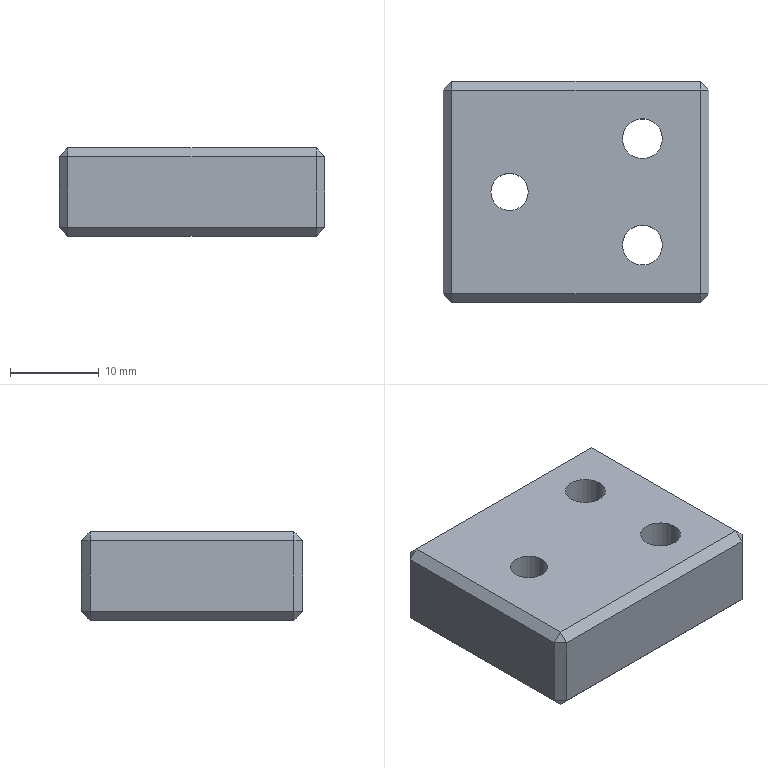Part | STEP file | 04-23 belt tensioning plate | 1 solid | 38 faces | box 30 x 25 x 10 mm | volume 6603 mm3 | plane 28 | cylinder 10 | commonest cylinder face diameters 4.5 x4 8 x4 4.2 x2
STEP:
#1=CARTESIAN_POINT('',(-9.6,0.,10.));
#2=VERTEX_POINT('',#1);
#3=CARTESIAN_POINT('',(-5.4,0.,10.));
#4=VERTEX_POINT('',#3);
#5=CARTESIAN_POINT('',(-7.5,0.,10.));
#6=DIRECTION('',(0.,0.,1.));
#7=DIRECTION('',(1.,0.,0.));
#8=AXIS2_PLACEMENT_3D('',#5,#6,#7);
#9=CIRCLE('',#8,2.1);
#10=EDGE_CURVE('',#2,#4,#9,.T.);
#11=ORIENTED_EDGE('',*,*,#10,.T.);
#12=CARTESIAN_POINT('',(-5.4,0.,0.));
#13=VERTEX_POINT('',#12);
#14=CARTESIAN_POINT('',(-5.4,0.,0.));
#15=DIRECTION('',(0.,0.,-1.));
#16=VECTOR('',#15,1000.);
#17=LINE('',#14,#16);
#18=EDGE_CURVE('',#4,#13,#17,.T.);
#19=ORIENTED_EDGE('',*,*,#18,.T.);
#20=CARTESIAN_POINT('',(-9.6,0.,0.));
#21=VERTEX_POINT('',#20);
#22=CARTESIAN_POINT('',(-7.5,0.,0.));
#23=DIRECTION('',(0.,0.,-1.));
#24=DIRECTION('',(-1.,0.,0.));
#25=AXIS2_PLACEMENT_3D('',#22,#23,#24);
#26=CIRCLE('',#25,2.1);
#27=EDGE_CURVE('',#13,#21,#26,.T.);
#28=ORIENTED_EDGE('',*,*,#27,.T.);
#29=CARTESIAN_POINT('',(-9.6,0.,0.));
#30=DIRECTION('',(0.,0.,-1.));
#31=VECTOR('',#30,1000.);
#32=LINE('',#29,#31);
#33=EDGE_CURVE('',#2,#21,#32,.T.);
#34=ORIENTED_EDGE('',*,*,#33,.F.);
#35=EDGE_LOOP('',(#11,#19,#28,#34));
#36=FACE_OUTER_BOUND('',#35,.T.);
#37=CARTESIAN_POINT('',(-7.5,0.,0.));
#38=DIRECTION('',(0.,0.,-1.));
#39=DIRECTION('',(-1.,0.,0.));
#40=AXIS2_PLACEMENT_3D('',#37,#38,#39);
#41=CYLINDRICAL_SURFACE('',#40,2.1);
#42=ADVANCED_FACE('',(#36),#41,.F.);
#43=CARTESIAN_POINT('',(11.5,6.,4.6));
#44=VERTEX_POINT('',#43);
#45=CARTESIAN_POINT('',(3.5,6.,4.6));
#46=VERTEX_POINT('',#45);
#47=CARTESIAN_POINT('',(7.5,6.,4.6));
#48=DIRECTION('',(0.,0.,-1.));
#49=DIRECTION('',(-1.,0.,0.));
#50=AXIS2_PLACEMENT_3D('',#47,#48,#49);
#51=CIRCLE('',#50,4.);
#52=EDGE_CURVE('',#44,#46,#51,.T.);
#53=ORIENTED_EDGE('',*,*,#52,.F.);
#54=CARTESIAN_POINT('',(11.5,6.,0.));
#55=VERTEX_POINT('',#54);
#56=CARTESIAN_POINT('',(11.5,6.,0.));
#57=DIRECTION('',(0.,0.,-1.));
#58=VECTOR('',#57,1000.);
#59=LINE('',#56,#58);
#60=EDGE_CURVE('',#44,#55,#59,.T.);
#61=ORIENTED_EDGE('',*,*,#60,.T.);
#62=CARTESIAN_POINT('',(3.5,6.,0.));
#63=VERTEX_POINT('',#62);
#64=CARTESIAN_POINT('',(7.5,6.,0.));
#65=DIRECTION('',(0.,0.,-1.));
#66=DIRECTION('',(-1.,0.,0.));
#67=AXIS2_PLACEMENT_3D('',#64,#65,#66);
#68=CIRCLE('',#67,4.);
#69=EDGE_CURVE('',#55,#63,#68,.T.);
#70=ORIENTED_EDGE('',*,*,#69,.T.);
#71=CARTESIAN_POINT('',(3.5,6.,0.));
#72=DIRECTION('',(0.,0.,-1.));
#73=VECTOR('',#72,1000.);
#74=LINE('',#71,#73);
#75=EDGE_CURVE('',#46,#63,#74,.T.);
#76=ORIENTED_EDGE('',*,*,#75,.F.);
#77=EDGE_LOOP('',(#53,#61,#70,#76));
#78=FACE_OUTER_BOUND('',#77,.T.);
#79=CARTESIAN_POINT('',(7.5,6.,0.));
#80=DIRECTION('',(0.,0.,-1.));
#81=DIRECTION('',(-1.,0.,0.));
#82=AXIS2_PLACEMENT_3D('',#79,#80,#81);
#83=CYLINDRICAL_SURFACE('',#82,4.);
#84=ADVANCED_FACE('',(#78),#83,.F.);
#85=CARTESIAN_POINT('',(9.75,6.,10.));
#86=VERTEX_POINT('',#85);
#87=CARTESIAN_POINT('',(5.25,6.,10.));
#88=VERTEX_POINT('',#87);
#89=CARTESIAN_POINT('',(7.5,6.,10.));
#90=DIRECTION('',(0.,0.,-1.));
#91=DIRECTION('',(-1.,0.,0.));
#92=AXIS2_PLACEMENT_3D('',#89,#90,#91);
#93=CIRCLE('',#92,2.25);
#94=EDGE_CURVE('',#86,#88,#93,.T.);
#95=ORIENTED_EDGE('',*,*,#94,.F.);
#96=CARTESIAN_POINT('',(9.75,6.,4.6));
#97=VERTEX_POINT('',#96);
#98=CARTESIAN_POINT('',(9.75,6.,0.));
#99=DIRECTION('',(0.,0.,-1.));
#100=VECTOR('',#99,1000.);
#101=LINE('',#98,#100);
#102=EDGE_CURVE('',#86,#97,#101,.T.);
#103=ORIENTED_EDGE('',*,*,#102,.T.);
#104=CARTESIAN_POINT('',(5.25,6.,4.6));
#105=VERTEX_POINT('',#104);
#106=CARTESIAN_POINT('',(7.5,6.,4.6));
#107=DIRECTION('',(0.,0.,-1.));
#108=DIRECTION('',(-1.,0.,0.));
#109=AXIS2_PLACEMENT_3D('',#106,#107,#108);
#110=CIRCLE('',#109,2.25);
#111=EDGE_CURVE('',#97,#105,#110,.T.);
#112=ORIENTED_EDGE('',*,*,#111,.T.);
#113=CARTESIAN_POINT('',(5.25,6.,0.));
#114=DIRECTION('',(0.,0.,-1.));
#115=VECTOR('',#114,1000.);
#116=LINE('',#113,#115);
#117=EDGE_CURVE('',#88,#105,#116,.T.);
#118=ORIENTED_EDGE('',*,*,#117,.F.);
#119=EDGE_LOOP('',(#95,#103,#112,#118));
#120=FACE_OUTER_BOUND('',#119,.T.);
#121=CARTESIAN_POINT('',(7.5,6.,0.));
#122=DIRECTION('',(0.,0.,-1.));
#123=DIRECTION('',(-1.,0.,0.));
#124=AXIS2_PLACEMENT_3D('',#121,#122,#123);
#125=CYLINDRICAL_SURFACE('',#124,2.25);
#126=ADVANCED_FACE('',(#120),#125,.F.);
#127=CARTESIAN_POINT('',(11.5,-6.,4.6));
#128=VERTEX_POINT('',#127);
#129=CARTESIAN_POINT('',(3.5,-6.,4.6));
#130=VERTEX_POINT('',#129);
#131=CARTESIAN_POINT('',(7.5,-6.,4.6));
#132=DIRECTION('',(0.,0.,-1.));
#133=DIRECTION('',(-1.,0.,0.));
#134=AXIS2_PLACEMENT_3D('',#131,#132,#133);
#135=CIRCLE('',#134,4.);
#136=EDGE_CURVE('',#128,#130,#135,.T.);
#137=ORIENTED_EDGE('',*,*,#136,.F.);
#138=CARTESIAN_POINT('',(11.5,-6.,0.));
#139=VERTEX_POINT('',#138);
#140=CARTESIAN_POINT('',(11.5,-6.,0.));
#141=DIRECTION('',(0.,0.,-1.));
#142=VECTOR('',#141,1000.);
#143=LINE('',#140,#142);
#144=EDGE_CURVE('',#128,#139,#143,.T.);
#145=ORIENTED_EDGE('',*,*,#144,.T.);
#146=CARTESIAN_POINT('',(3.5,-6.,0.));
#147=VERTEX_POINT('',#146);
#148=CARTESIAN_POINT('',(7.5,-6.,0.));
#149=DIRECTION('',(0.,0.,-1.));
#150=DIRECTION('',(-1.,0.,0.));
#151=AXIS2_PLACEMENT_3D('',#148,#149,#150);
#152=CIRCLE('',#151,4.);
#153=EDGE_CURVE('',#139,#147,#152,.T.);
#154=ORIENTED_EDGE('',*,*,#153,.T.);
#155=CARTESIAN_POINT('',(3.5,-6.,0.));
#156=DIRECTION('',(0.,0.,-1.));
#157=VECTOR('',#156,1000.);
#158=LINE('',#155,#157);
#159=EDGE_CURVE('',#130,#147,#158,.T.);
#160=ORIENTED_EDGE('',*,*,#159,.F.);
#161=EDGE_LOOP('',(#137,#145,#154,#160));
#162=FACE_OUTER_BOUND('',#161,.T.);
#163=CARTESIAN_POINT('',(7.5,-6.,0.));
#164=DIRECTION('',(0.,0.,-1.));
#165=DIRECTION('',(-1.,0.,0.));
#166=AXIS2_PLACEMENT_3D('',#163,#164,#165);
#167=CYLINDRICAL_SURFACE('',#166,4.);
#168=ADVANCED_FACE('',(#162),#167,.F.);
#169=CARTESIAN_POINT('',(9.75,-6.,10.));
#170=VERTEX_POINT('',#169);
#171=CARTESIAN_POINT('',(5.25,-6.,10.));
#172=VERTEX_POINT('',#171);
#173=CARTESIAN_POINT('',(7.5,-6.,10.));
#174=DIRECTION('',(0.,0.,-1.));
#175=DIRECTION('',(-1.,0.,0.));
#176=AXIS2_PLACEMENT_3D('',#173,#174,#175);
#177=CIRCLE('',#176,2.25);
#178=EDGE_CURVE('',#170,#172,#177,.T.);
#179=ORIENTED_EDGE('',*,*,#178,.F.);
#180=CARTESIAN_POINT('',(9.75,-6.,4.6));
#181=VERTEX_POINT('',#180);
#182=CARTESIAN_POINT('',(9.75,-6.,0.));
#183=DIRECTION('',(0.,0.,-1.));
#184=VECTOR('',#183,1000.);
#185=LINE('',#182,#184);
#186=EDGE_CURVE('',#170,#181,#185,.T.);
#187=ORIENTED_EDGE('',*,*,#186,.T.);
#188=CARTESIAN_POINT('',(5.25,-6.,4.6));
#189=VERTEX_POINT('',#188);
#190=CARTESIAN_POINT('',(7.5,-6.,4.6));
#191=DIRECTION('',(0.,0.,-1.));
#192=DIRECTION('',(-1.,0.,0.));
#193=AXIS2_PLACEMENT_3D('',#190,#191,#192);
#194=CIRCLE('',#193,2.25);
#195=EDGE_CURVE('',#181,#189,#194,.T.);
#196=ORIENTED_EDGE('',*,*,#195,.T.);
#197=CARTESIAN_POINT('',(5.25,-6.,0.));
#198=DIRECTION('',(0.,0.,-1.));
#199=VECTOR('',#198,1000.);
#200=LINE('',#197,#199);
#201=EDGE_CURVE('',#172,#189,#200,.T.);
#202=ORIENTED_EDGE('',*,*,#201,.F.);
#203=EDGE_LOOP('',(#179,#187,#196,#202));
#204=FACE_OUTER_BOUND('',#203,.T.);
#205=CARTESIAN_POINT('',(7.5,-6.,0.));
#206=DIRECTION('',(0.,0.,-1.));
#207=DIRECTION('',(-1.,0.,0.));
#208=AXIS2_PLACEMENT_3D('',#205,#206,#207);
#209=CYLINDRICAL_SURFACE('',#208,2.25);
#210=ADVANCED_FACE('',(#204),#209,.F.);
#211=CARTESIAN_POINT('',(15.,11.5,9.));
#212=VERTEX_POINT('',#211);
#213=CARTESIAN_POINT('',(15.,-11.5,9.));
#214=VERTEX_POINT('',#213);
#215=CARTESIAN_POINT('',(15.,-12.5,9.));
#216=DIRECTION('',(0.,-1.,0.));
#217=VECTOR('',#216,1000.);
#218=LINE('',#215,#217);
#219=EDGE_CURVE('',#212,#214,#218,.T.);
#220=ORIENTED_EDGE('',*,*,#219,.T.);
#221=CARTESIAN_POINT('',(15.,-11.5,1.));
#222=VERTEX_POINT('',#221);
#223=CARTESIAN_POINT('',(15.,-11.5,10.));
#224=DIRECTION('',(0.,0.,-1.));
#225=VECTOR('',#224,1000.);
#226=LINE('',#223,#225);
#227=EDGE_CURVE('',#214,#222,#226,.T.);
#228=ORIENTED_EDGE('',*,*,#227,.T.);
#229=CARTESIAN_POINT('',(15.,11.5,1.));
#230=VERTEX_POINT('',#229);
#231=CARTESIAN_POINT('',(15.,12.5,1.));
#232=DIRECTION('',(0.,1.,0.));
#233=VECTOR('',#232,1000.);
#234=LINE('',#231,#233);
#235=EDGE_CURVE('',#222,#230,#234,.T.);
#236=ORIENTED_EDGE('',*,*,#235,.T.);
#237=CARTESIAN_POINT('',(15.,11.5,10.));
#238=DIRECTION('',(0.,0.,1.));
#239=VECTOR('',#238,1000.);
#240=LINE('',#237,#239);
#241=EDGE_CURVE('',#230,#212,#240,.T.);
#242=ORIENTED_EDGE('',*,*,#241,.T.);
#243=EDGE_LOOP('',(#220,#228,#236,#242));
#244=FACE_OUTER_BOUND('',#243,.T.);
#245=CARTESIAN_POINT('',(15.,12.5,10.));
#246=DIRECTION('',(-1.,0.,0.));
#247=DIRECTION('',(0.,-1.,0.));
#248=AXIS2_PLACEMENT_3D('',#245,#246,#247);
#249=PLANE('',#248);
#250=ADVANCED_FACE('',(#244),#249,.F.);
#251=CARTESIAN_POINT('',(-14.,12.5,9.));
#252=VERTEX_POINT('',#251);
#253=CARTESIAN_POINT('',(14.,12.5,9.));
#254=VERTEX_POINT('',#253);
#255=CARTESIAN_POINT('',(15.,12.5,9.));
#256=DIRECTION('',(1.,0.,0.));
#257=VECTOR('',#256,1000.);
#258=LINE('',#255,#257);
#259=EDGE_CURVE('',#252,#254,#258,.T.);
#260=ORIENTED_EDGE('',*,*,#259,.T.);
#261=CARTESIAN_POINT('',(14.,12.5,1.));
#262=VERTEX_POINT('',#261);
#263=CARTESIAN_POINT('',(14.,12.5,10.));
#264=DIRECTION('',(0.,0.,-1.));
#265=VECTOR('',#264,1000.);
#266=LINE('',#263,#265);
#267=EDGE_CURVE('',#254,#262,#266,.T.);
#268=ORIENTED_EDGE('',*,*,#267,.T.);
#269=CARTESIAN_POINT('',(-14.,12.5,1.));
#270=VERTEX_POINT('',#269);
#271=CARTESIAN_POINT('',(-15.,12.5,1.));
#272=DIRECTION('',(-1.,0.,0.));
#273=VECTOR('',#272,1000.);
#274=LINE('',#271,#273);
#275=EDGE_CURVE('',#262,#270,#274,.T.);
#276=ORIENTED_EDGE('',*,*,#275,.T.);
#277=CARTESIAN_POINT('',(-14.,12.5,10.));
#278=DIRECTION('',(0.,0.,1.));
#279=VECTOR('',#278,1000.);
#280=LINE('',#277,#279);
#281=EDGE_CURVE('',#270,#252,#280,.T.);
#282=ORIENTED_EDGE('',*,*,#281,.T.);
#283=EDGE_LOOP('',(#260,#268,#276,#282));
#284=FACE_OUTER_BOUND('',#283,.T.);
#285=CARTESIAN_POINT('',(-15.,12.5,10.));
#286=DIRECTION('',(0.,-1.,0.));
#287=DIRECTION('',(0.,0.,-1.));
#288=AXIS2_PLACEMENT_3D('',#285,#286,#287);
#289=PLANE('',#288);
#290=ADVANCED_FACE('',(#284),#289,.F.);
#291=CARTESIAN_POINT('',(-15.,-11.5,1.));
#292=VERTEX_POINT('',#291);
#293=CARTESIAN_POINT('',(-15.,-11.5,9.));
#294=VERTEX_POINT('',#293);
#295=CARTESIAN_POINT('',(-15.,-11.5,10.));
#296=DIRECTION('',(0.,0.,1.));
#297=VECTOR('',#296,1000.);
#298=LINE('',#295,#297);
#299=EDGE_CURVE('',#292,#294,#298,.T.);
#300=ORIENTED_EDGE('',*,*,#299,.T.);
#301=CARTESIAN_POINT('',(-15.,11.5,9.));
#302=VERTEX_POINT('',#301);
#303=CARTESIAN_POINT('',(-15.,12.5,9.));
#304=DIRECTION('',(0.,1.,0.));
#305=VECTOR('',#304,1000.);
#306=LINE('',#303,#305);
#307=EDGE_CURVE('',#294,#302,#306,.T.);
#308=ORIENTED_EDGE('',*,*,#307,.T.);
#309=CARTESIAN_POINT('',(-15.,11.5,1.));
#310=VERTEX_POINT('',#309);
#311=CARTESIAN_POINT('',(-15.,11.5,10.));
#312=DIRECTION('',(0.,0.,-1.));
#313=VECTOR('',#312,1000.);
#314=LINE('',#311,#313);
#315=EDGE_CURVE('',#302,#310,#314,.T.);
#316=ORIENTED_EDGE('',*,*,#315,.T.);
#317=CARTESIAN_POINT('',(-15.,12.5,1.));
#318=DIRECTION('',(0.,-1.,0.));
#319=VECTOR('',#318,1000.);
#320=LINE('',#317,#319);
#321=EDGE_CURVE('',#310,#292,#320,.T.);
#322=ORIENTED_EDGE('',*,*,#321,.T.);
#323=EDGE_LOOP('',(#300,#308,#316,#322));
#324=FACE_OUTER_BOUND('',#323,.T.);
#325=CARTESIAN_POINT('',(-15.,12.5,10.));
#326=DIRECTION('',(1.,0.,0.));
#327=DIRECTION('',(0.,1.,0.));
#328=AXIS2_PLACEMENT_3D('',#325,#326,#327);
#329=PLANE('',#328);
#330=ADVANCED_FACE('',(#324),#329,.F.);
#331=CARTESIAN_POINT('',(14.,-12.5,1.));
#332=VERTEX_POINT('',#331);
#333=CARTESIAN_POINT('',(14.,-12.5,9.));
#334=VERTEX_POINT('',#333);
#335=CARTESIAN_POINT('',(14.,-12.5,10.));
#336=DIRECTION('',(0.,0.,1.));
#337=VECTOR('',#336,1000.);
#338=LINE('',#335,#337);
#339=EDGE_CURVE('',#332,#334,#338,.T.);
#340=ORIENTED_EDGE('',*,*,#339,.T.);
#341=CARTESIAN_POINT('',(-14.,-12.5,9.));
#342=VERTEX_POINT('',#341);
#343=CARTESIAN_POINT('',(-15.,-12.5,9.));
#344=DIRECTION('',(-1.,0.,0.));
#345=VECTOR('',#344,1000.);
#346=LINE('',#343,#345);
#347=EDGE_CURVE('',#334,#342,#346,.T.);
#348=ORIENTED_EDGE('',*,*,#347,.T.);
#349=CARTESIAN_POINT('',(-14.,-12.5,1.));
#350=VERTEX_POINT('',#349);
#351=CARTESIAN_POINT('',(-14.,-12.5,10.));
#352=DIRECTION('',(0.,0.,-1.));
#353=VECTOR('',#352,1000.);
#354=LINE('',#351,#353);
#355=EDGE_CURVE('',#342,#350,#354,.T.);
#356=ORIENTED_EDGE('',*,*,#355,.T.);
#357=CARTESIAN_POINT('',(-15.,-12.5,1.));
#358=DIRECTION('',(1.,0.,0.));
#359=VECTOR('',#358,1000.);
#360=LINE('',#357,#359);
#361=EDGE_CURVE('',#350,#332,#360,.T.);
#362=ORIENTED_EDGE('',*,*,#361,.T.);
#363=EDGE_LOOP('',(#340,#348,#356,#362));
#364=FACE_OUTER_BOUND('',#363,.T.);
#365=CARTESIAN_POINT('',(-15.,-12.5,10.));
#366=DIRECTION('',(0.,1.,0.));
#367=DIRECTION('',(0.,0.,1.));
#368=AXIS2_PLACEMENT_3D('',#365,#366,#367);
#369=PLANE('',#368);
#370=ADVANCED_FACE('',(#364),#369,.F.);
#371=ORIENTED_EDGE('',*,*,#10,.F.);
#372=CARTESIAN_POINT('',(-7.5,0.,10.));
#373=DIRECTION('',(0.,0.,1.));
#374=DIRECTION('',(1.,0.,0.));
#375=AXIS2_PLACEMENT_3D('',#372,#373,#374);
#376=CIRCLE('',#375,2.1);
#377=EDGE_CURVE('',#4,#2,#376,.T.);
#378=ORIENTED_EDGE('',*,*,#377,.F.);
#379=EDGE_LOOP('',(#371,#378));
#380=FACE_BOUND('',#379,.T.);
#381=CARTESIAN_POINT('',(7.5,6.,10.));
#382=DIRECTION('',(0.,0.,-1.));
#383=DIRECTION('',(-1.,0.,0.));
#384=AXIS2_PLACEMENT_3D('',#381,#382,#383);
#385=CIRCLE('',#384,2.25);
#386=EDGE_CURVE('',#88,#86,#385,.T.);
#387=ORIENTED_EDGE('',*,*,#386,.T.);
#388=ORIENTED_EDGE('',*,*,#94,.T.);
#389=EDGE_LOOP('',(#387,#388));
#390=FACE_BOUND('',#389,.T.);
#391=CARTESIAN_POINT('',(7.5,-6.,10.));
#392=DIRECTION('',(0.,0.,-1.));
#393=DIRECTION('',(-1.,0.,0.));
#394=AXIS2_PLACEMENT_3D('',#391,#392,#393);
#395=CIRCLE('',#394,2.25);
#396=EDGE_CURVE('',#172,#170,#395,.T.);
#397=ORIENTED_EDGE('',*,*,#396,.T.);
#398=ORIENTED_EDGE('',*,*,#178,.T.);
#399=EDGE_LOOP('',(#397,#398));
#400=FACE_BOUND('',#399,.T.);
#401=CARTESIAN_POINT('',(-14.,-11.5,10.));
#402=VERTEX_POINT('',#401);
#403=CARTESIAN_POINT('',(14.,-11.5,10.));
#404=VERTEX_POINT('',#403);
#405=CARTESIAN_POINT('',(15.,-11.5,10.));
#406=DIRECTION('',(1.,0.,0.));
#407=VECTOR('',#406,1000.);
#408=LINE('',#405,#407);
#409=EDGE_CURVE('',#402,#404,#408,.T.);
#410=ORIENTED_EDGE('',*,*,#409,.T.);
#411=CARTESIAN_POINT('',(14.,11.5,10.));
#412=VERTEX_POINT('',#411);
#413=CARTESIAN_POINT('',(14.,12.5,10.));
#414=DIRECTION('',(0.,1.,0.));
#415=VECTOR('',#414,1000.);
#416=LINE('',#413,#415);
#417=EDGE_CURVE('',#404,#412,#416,.T.);
#418=ORIENTED_EDGE('',*,*,#417,.T.);
#419=CARTESIAN_POINT('',(-14.,11.5,10.));
#420=VERTEX_POINT('',#419);
#421=CARTESIAN_POINT('',(-15.,11.5,10.));
#422=DIRECTION('',(-1.,0.,0.));
#423=VECTOR('',#422,1000.);
#424=LINE('',#421,#423);
#425=EDGE_CURVE('',#412,#420,#424,.T.);
#426=ORIENTED_EDGE('',*,*,#425,.T.);
#427=CARTESIAN_POINT('',(-14.,-12.5,10.));
#428=DIRECTION('',(0.,-1.,0.));
#429=VECTOR('',#428,1000.);
#430=LINE('',#427,#429);
#431=EDGE_CURVE('',#420,#402,#430,.T.);
#432=ORIENTED_EDGE('',*,*,#431,.T.);
#433=EDGE_LOOP('',(#410,#418,#426,#432));
#434=FACE_OUTER_BOUND('',#433,.T.);
#435=CARTESIAN_POINT('',(15.,-12.5,10.));
#436=DIRECTION('',(0.,0.,1.));
#437=DIRECTION('',(1.,0.,0.));
#438=AXIS2_PLACEMENT_3D('',#435,#436,#437);
#439=PLANE('',#438);
#440=ADVANCED_FACE('',(#380,#390,#400,#434),#439,.T.);
#441=CARTESIAN_POINT('',(-7.5,0.,0.));
#442=DIRECTION('',(0.,0.,-1.));
#443=DIRECTION('',(-1.,0.,0.));
#444=AXIS2_PLACEMENT_3D('',#441,#442,#443);
#445=CIRCLE('',#444,2.1);
#446=EDGE_CURVE('',#21,#13,#445,.T.);
#447=ORIENTED_EDGE('',*,*,#446,.F.);
#448=ORIENTED_EDGE('',*,*,#27,.F.);
#449=EDGE_LOOP('',(#447,#448));
#450=FACE_BOUND('',#449,.T.);
#451=CARTESIAN_POINT('',(7.5,6.,0.));
#452=DIRECTION('',(0.,0.,-1.));
#453=DIRECTION('',(-1.,0.,0.));
#454=AXIS2_PLACEMENT_3D('',#451,#452,#453);
#455=CIRCLE('',#454,4.);
#456=EDGE_CURVE('',#63,#55,#455,.T.);
#457=ORIENTED_EDGE('',*,*,#456,.F.);
#458=ORIENTED_EDGE('',*,*,#69,.F.);
#459=EDGE_LOOP('',(#457,#458));
#460=FACE_BOUND('',#459,.T.);
#461=CARTESIAN_POINT('',(7.5,-6.,0.));
#462=DIRECTION('',(0.,0.,-1.));
#463=DIRECTION('',(-1.,0.,0.));
#464=AXIS2_PLACEMENT_3D('',#461,#462,#463);
#465=CIRCLE('',#464,4.);
#466=EDGE_CURVE('',#147,#139,#465,.T.);
#467=ORIENTED_EDGE('',*,*,#466,.F.);
#468=ORIENTED_EDGE('',*,*,#153,.F.);
#469=EDGE_LOOP('',(#467,#468));
#470=FACE_BOUND('',#469,.T.);
#471=CARTESIAN_POINT('',(-14.,11.5,0.));
#472=VERTEX_POINT('',#471);
#473=CARTESIAN_POINT('',(14.,11.5,0.));
#474=VERTEX_POINT('',#473);
#475=CARTESIAN_POINT('',(15.,11.5,0.));
#476=DIRECTION('',(1.,0.,0.));
#477=VECTOR('',#476,1000.);
#478=LINE('',#475,#477);
#479=EDGE_CURVE('',#472,#474,#478,.T.);
#480=ORIENTED_EDGE('',*,*,#479,.T.);
#481=CARTESIAN_POINT('',(14.,-11.5,0.));
#482=VERTEX_POINT('',#481);
#483=CARTESIAN_POINT('',(14.,-12.5,0.));
#484=DIRECTION('',(0.,-1.,0.));
#485=VECTOR('',#484,1000.);
#486=LINE('',#483,#485);
#487=EDGE_CURVE('',#474,#482,#486,.T.);
#488=ORIENTED_EDGE('',*,*,#487,.T.);
#489=CARTESIAN_POINT('',(-14.,-11.5,0.));
#490=VERTEX_POINT('',#489);
#491=CARTESIAN_POINT('',(15.,-11.5,0.));
#492=DIRECTION('',(-1.,0.,0.));
#493=VECTOR('',#492,1000.);
#494=LINE('',#491,#493);
#495=EDGE_CURVE('',#482,#490,#494,.T.);
#496=ORIENTED_EDGE('',*,*,#495,.T.);
#497=CARTESIAN_POINT('',(-14.,-12.5,0.));
#498=DIRECTION('',(0.,1.,0.));
#499=VECTOR('',#498,1000.);
#500=LINE('',#497,#499);
#501=EDGE_CURVE('',#490,#472,#500,.T.);
#502=ORIENTED_EDGE('',*,*,#501,.T.);
#503=EDGE_LOOP('',(#480,#488,#496,#502));
#504=FACE_OUTER_BOUND('',#503,.T.);
#505=CARTESIAN_POINT('',(15.,-12.5,0.));
#506=DIRECTION('',(0.,0.,1.));
#507=DIRECTION('',(1.,0.,0.));
#508=AXIS2_PLACEMENT_3D('',#505,#506,#507);
#509=PLANE('',#508);
#510=ADVANCED_FACE('',(#450,#460,#470,#504),#509,.F.);
#511=CARTESIAN_POINT('',(-14.,-11.5,0.));
#512=DIRECTION('',(0.7071,0.,-0.7071));
#513=VECTOR('',#512,1000.);
#514=LINE('',#511,#513);
#515=EDGE_CURVE('',#292,#490,#514,.T.);
#516=ORIENTED_EDGE('',*,*,#515,.F.);
#517=ORIENTED_EDGE('',*,*,#321,.F.);
#518=CARTESIAN_POINT('',(-14.,11.5,0.));
#519=DIRECTION('',(-0.7071,0.,0.7071));
#520=VECTOR('',#519,1000.);
#521=LINE('',#518,#520);
#522=EDGE_CURVE('',#472,#310,#521,.T.);
#523=ORIENTED_EDGE('',*,*,#522,.F.);
#524=ORIENTED_EDGE('',*,*,#501,.F.);
#525=EDGE_LOOP('',(#516,#517,#523,#524));
#526=FACE_OUTER_BOUND('',#525,.T.);
#527=CARTESIAN_POINT('',(-15.,12.5,1.));
#528=DIRECTION('',(0.7071,0.,0.7071));
#529=DIRECTION('',(0.7071,0.,-0.7071));
#530=AXIS2_PLACEMENT_3D('',#527,#528,#529);
#531=PLANE('',#530);
#532=ADVANCED_FACE('',(#526),#531,.F.);
#533=CARTESIAN_POINT('',(-14.5,-12.,1.));
#534=DIRECTION('',(0.7071,-0.7071,0.));
#535=VECTOR('',#534,1000.);
#536=LINE('',#533,#535);
#537=EDGE_CURVE('',#292,#350,#536,.T.);
#538=ORIENTED_EDGE('',*,*,#537,.F.);
#539=ORIENTED_EDGE('',*,*,#515,.T.);
#540=CARTESIAN_POINT('',(-14.,-11.5,0.));
#541=DIRECTION('',(0.,0.7071,-0.7071));
#542=VECTOR('',#541,1000.);
#543=LINE('',#540,#542);
#544=EDGE_CURVE('',#350,#490,#543,.T.);
#545=ORIENTED_EDGE('',*,*,#544,.F.);
#546=EDGE_LOOP('',(#538,#539,#545));
#547=FACE_OUTER_BOUND('',#546,.T.);
#548=CARTESIAN_POINT('',(-14.,-11.5,0.));
#549=DIRECTION('',(-0.5774,-0.5774,-0.5774));
#550=DIRECTION('',(-0.7071,0.,0.7071));
#551=AXIS2_PLACEMENT_3D('',#548,#549,#550);
#552=PLANE('',#551);
#553=ADVANCED_FACE('',(#547),#552,.T.);
#554=CARTESIAN_POINT('',(-14.,11.5,0.));
#555=DIRECTION('',(0.,0.7071,0.7071));
#556=VECTOR('',#555,1000.);
#557=LINE('',#554,#556);
#558=EDGE_CURVE('',#472,#270,#557,.T.);
#559=ORIENTED_EDGE('',*,*,#558,.F.);
#560=ORIENTED_EDGE('',*,*,#522,.T.);
#561=CARTESIAN_POINT('',(-14.5,12.,1.));
#562=DIRECTION('',(-0.7071,-0.7071,0.));
#563=VECTOR('',#562,1000.);
#564=LINE('',#561,#563);
#565=EDGE_CURVE('',#270,#310,#564,.T.);
#566=ORIENTED_EDGE('',*,*,#565,.F.);
#567=EDGE_LOOP('',(#559,#560,#566));
#568=FACE_OUTER_BOUND('',#567,.T.);
#569=CARTESIAN_POINT('',(-14.,11.5,0.));
#570=DIRECTION('',(-0.5774,0.5774,-0.5774));
#571=DIRECTION('',(-0.7071,0.,0.7071));
#572=AXIS2_PLACEMENT_3D('',#569,#570,#571);
#573=PLANE('',#572);
#574=ADVANCED_FACE('',(#568),#573,.T.);
#575=ORIENTED_EDGE('',*,*,#544,.T.);
#576=ORIENTED_EDGE('',*,*,#495,.F.);
#577=CARTESIAN_POINT('',(14.,-11.5,0.));
#578=DIRECTION('',(0.,0.7071,-0.7071));
#579=VECTOR('',#578,1000.);
#580=LINE('',#577,#579);
#581=EDGE_CURVE('',#332,#482,#580,.T.);
#582=ORIENTED_EDGE('',*,*,#581,.F.);
#583=ORIENTED_EDGE('',*,*,#361,.F.);
#584=EDGE_LOOP('',(#575,#576,#582,#583));
#585=FACE_OUTER_BOUND('',#584,.T.);
#586=CARTESIAN_POINT('',(-15.,-12.5,1.));
#587=DIRECTION('',(0.,0.7071,0.7071));
#588=DIRECTION('',(0.,-0.7071,0.7071));
#589=AXIS2_PLACEMENT_3D('',#586,#587,#588);
#590=PLANE('',#589);
#591=ADVANCED_FACE('',(#585),#590,.F.);
#592=ORIENTED_EDGE('',*,*,#537,.T.);
#593=ORIENTED_EDGE('',*,*,#355,.F.);
#594=CARTESIAN_POINT('',(-14.,-12.5,9.));
#595=DIRECTION('',(0.7071,-0.7071,0.));
#596=VECTOR('',#595,1000.);
#597=LINE('',#594,#596);
#598=EDGE_CURVE('',#294,#342,#597,.T.);
#599=ORIENTED_EDGE('',*,*,#598,.F.);
#600=ORIENTED_EDGE('',*,*,#299,.F.);
#601=EDGE_LOOP('',(#592,#593,#599,#600));
#602=FACE_OUTER_BOUND('',#601,.T.);
#603=CARTESIAN_POINT('',(-14.,-12.5,10.));
#604=DIRECTION('',(0.7071,0.7071,0.));
#605=DIRECTION('',(-0.7071,0.7071,0.));
#606=AXIS2_PLACEMENT_3D('',#603,#604,#605);
#607=PLANE('',#606);
#608=ADVANCED_FACE('',(#602),#607,.F.);
#609=CARTESIAN_POINT('',(-15.,11.5,9.));
#610=DIRECTION('',(0.7071,0.,0.7071));
#611=VECTOR('',#610,1000.);
#612=LINE('',#609,#611);
#613=EDGE_CURVE('',#302,#420,#612,.T.);
#614=ORIENTED_EDGE('',*,*,#613,.F.);
#615=ORIENTED_EDGE('',*,*,#307,.F.);
#616=CARTESIAN_POINT('',(-14.5,-11.5,9.5));
#617=DIRECTION('',(-0.7071,0.,-0.7071));
#618=VECTOR('',#617,1000.);
#619=LINE('',#616,#618);
#620=EDGE_CURVE('',#402,#294,#619,.T.);
#621=ORIENTED_EDGE('',*,*,#620,.F.);
#622=ORIENTED_EDGE('',*,*,#431,.F.);
#623=EDGE_LOOP('',(#614,#615,#621,#622));
#624=FACE_OUTER_BOUND('',#623,.T.);
#625=CARTESIAN_POINT('',(-14.,-12.5,10.));
#626=DIRECTION('',(-0.7071,0.,0.7071));
#627=DIRECTION('',(0.7071,0.,0.7071));
#628=AXIS2_PLACEMENT_3D('',#625,#626,#627);
#629=PLANE('',#628);
#630=ADVANCED_FACE('',(#624),#629,.T.);
#631=ORIENTED_EDGE('',*,*,#565,.T.);
#632=ORIENTED_EDGE('',*,*,#315,.F.);
#633=CARTESIAN_POINT('',(-15.,11.5,9.));
#634=DIRECTION('',(-0.7071,-0.7071,0.));
#635=VECTOR('',#634,1000.);
#636=LINE('',#633,#635);
#637=EDGE_CURVE('',#252,#302,#636,.T.);
#638=ORIENTED_EDGE('',*,*,#637,.F.);
#639=ORIENTED_EDGE('',*,*,#281,.F.);
#640=EDGE_LOOP('',(#631,#632,#638,#639));
#641=FACE_OUTER_BOUND('',#640,.T.);
#642=CARTESIAN_POINT('',(-15.,11.5,10.));
#643=DIRECTION('',(0.7071,-0.7071,0.));
#644=DIRECTION('',(0.7071,0.7071,0.));
#645=AXIS2_PLACEMENT_3D('',#642,#643,#644);
#646=PLANE('',#645);
#647=ADVANCED_FACE('',(#641),#646,.F.);
#648=ORIENTED_EDGE('',*,*,#558,.T.);
#649=ORIENTED_EDGE('',*,*,#275,.F.);
#650=CARTESIAN_POINT('',(14.,12.,0.5));
#651=DIRECTION('',(0.,0.7071,0.7071));
#652=VECTOR('',#651,1000.);
#653=LINE('',#650,#652);
#654=EDGE_CURVE('',#474,#262,#653,.T.);
#655=ORIENTED_EDGE('',*,*,#654,.F.);
#656=ORIENTED_EDGE('',*,*,#479,.F.);
#657=EDGE_LOOP('',(#648,#649,#655,#656));
#658=FACE_OUTER_BOUND('',#657,.T.);
#659=CARTESIAN_POINT('',(-15.,12.5,1.));
#660=DIRECTION('',(0.,-0.7071,0.7071));
#661=DIRECTION('',(0.,-0.7071,-0.7071));
#662=AXIS2_PLACEMENT_3D('',#659,#660,#661);
#663=PLANE('',#662);
#664=ADVANCED_FACE('',(#658),#663,.F.);
#665=CARTESIAN_POINT('',(14.,-11.5,0.));
#666=DIRECTION('',(0.7071,0.,0.7071));
#667=VECTOR('',#666,1000.);
#668=LINE('',#665,#667);
#669=EDGE_CURVE('',#482,#222,#668,.T.);
#670=ORIENTED_EDGE('',*,*,#669,.F.);
#671=ORIENTED_EDGE('',*,*,#487,.F.);
#672=CARTESIAN_POINT('',(15.,11.5,1.));
#673=DIRECTION('',(-0.7071,0.,-0.7071));
#674=VECTOR('',#673,1000.);
#675=LINE('',#672,#674);
#676=EDGE_CURVE('',#230,#474,#675,.T.);
#677=ORIENTED_EDGE('',*,*,#676,.F.);
#678=ORIENTED_EDGE('',*,*,#235,.F.);
#679=EDGE_LOOP('',(#670,#671,#677,#678));
#680=FACE_OUTER_BOUND('',#679,.T.);
#681=CARTESIAN_POINT('',(15.,12.5,1.));
#682=DIRECTION('',(-0.7071,0.,0.7071));
#683=DIRECTION('',(0.7071,0.,0.7071));
#684=AXIS2_PLACEMENT_3D('',#681,#682,#683);
#685=PLANE('',#684);
#686=ADVANCED_FACE('',(#680),#685,.F.);
#687=ORIENTED_EDGE('',*,*,#581,.T.);
#688=ORIENTED_EDGE('',*,*,#669,.T.);
#689=CARTESIAN_POINT('',(14.5,-12.,1.));
#690=DIRECTION('',(0.7071,0.7071,0.));
#691=VECTOR('',#690,1000.);
#692=LINE('',#689,#691);
#693=EDGE_CURVE('',#332,#222,#692,.T.);
#694=ORIENTED_EDGE('',*,*,#693,.F.);
#695=EDGE_LOOP('',(#687,#688,#694));
#696=FACE_OUTER_BOUND('',#695,.T.);
#697=CARTESIAN_POINT('',(14.,-11.5,0.));
#698=DIRECTION('',(0.5774,-0.5774,-0.5774));
#699=DIRECTION('',(0.,0.7071,-0.7071));
#700=AXIS2_PLACEMENT_3D('',#697,#698,#699);
#701=PLANE('',#700);
#702=ADVANCED_FACE('',(#696),#701,.T.);
#703=ORIENTED_EDGE('',*,*,#620,.T.);
#704=ORIENTED_EDGE('',*,*,#598,.T.);
#705=CARTESIAN_POINT('',(-14.,-12.5,9.));
#706=DIRECTION('',(0.,-0.7071,-0.7071));
#707=VECTOR('',#706,1000.);
#708=LINE('',#705,#707);
#709=EDGE_CURVE('',#402,#342,#708,.T.);
#710=ORIENTED_EDGE('',*,*,#709,.F.);
#711=EDGE_LOOP('',(#703,#704,#710));
#712=FACE_OUTER_BOUND('',#711,.T.);
#713=CARTESIAN_POINT('',(-14.,-12.5,9.));
#714=DIRECTION('',(-0.5774,-0.5774,0.5774));
#715=DIRECTION('',(0.7071,-0.7071,0.));
#716=AXIS2_PLACEMENT_3D('',#713,#714,#715);
#717=PLANE('',#716);
#718=ADVANCED_FACE('',(#712),#717,.T.);
#719=ORIENTED_EDGE('',*,*,#637,.T.);
#720=ORIENTED_EDGE('',*,*,#613,.T.);
#721=CARTESIAN_POINT('',(-14.,12.,9.5));
#722=DIRECTION('',(0.,-0.7071,0.7071));
#723=VECTOR('',#722,1000.);
#724=LINE('',#721,#723);
#725=EDGE_CURVE('',#252,#420,#724,.T.);
#726=ORIENTED_EDGE('',*,*,#725,.F.);
#727=EDGE_LOOP('',(#719,#720,#726));
#728=FACE_OUTER_BOUND('',#727,.T.);
#729=CARTESIAN_POINT('',(-15.,11.5,9.));
#730=DIRECTION('',(-0.5774,0.5774,0.5774));
#731=DIRECTION('',(0.7071,0.,0.7071));
#732=AXIS2_PLACEMENT_3D('',#729,#730,#731);
#733=PLANE('',#732);
#734=ADVANCED_FACE('',(#728),#733,.T.);
#735=ORIENTED_EDGE('',*,*,#676,.T.);
#736=ORIENTED_EDGE('',*,*,#654,.T.);
#737=CARTESIAN_POINT('',(15.,11.5,1.));
#738=DIRECTION('',(-0.7071,0.7071,0.));
#739=VECTOR('',#738,1000.);
#740=LINE('',#737,#739);
#741=EDGE_CURVE('',#230,#262,#740,.T.);
#742=ORIENTED_EDGE('',*,*,#741,.F.);
#743=EDGE_LOOP('',(#735,#736,#742));
#744=FACE_OUTER_BOUND('',#743,.T.);
#745=CARTESIAN_POINT('',(15.,11.5,1.));
#746=DIRECTION('',(0.5774,0.5774,-0.5774));
#747=DIRECTION('',(-0.7071,0.,-0.7071));
#748=AXIS2_PLACEMENT_3D('',#745,#746,#747);
#749=PLANE('',#748);
#750=ADVANCED_FACE('',(#744),#749,.T.);
#751=ORIENTED_EDGE('',*,*,#693,.T.);
#752=ORIENTED_EDGE('',*,*,#227,.F.);
#753=CARTESIAN_POINT('',(15.,-11.5,9.));
#754=DIRECTION('',(0.7071,0.7071,0.));
#755=VECTOR('',#754,1000.);
#756=LINE('',#753,#755);
#757=EDGE_CURVE('',#334,#214,#756,.T.);
#758=ORIENTED_EDGE('',*,*,#757,.F.);
#759=ORIENTED_EDGE('',*,*,#339,.F.);
#760=EDGE_LOOP('',(#751,#752,#758,#759));
#761=FACE_OUTER_BOUND('',#760,.T.);
#762=CARTESIAN_POINT('',(15.,-11.5,10.));
#763=DIRECTION('',(-0.7071,0.7071,0.));
#764=DIRECTION('',(-0.7071,-0.7071,0.));
#765=AXIS2_PLACEMENT_3D('',#762,#763,#764);
#766=PLANE('',#765);
#767=ADVANCED_FACE('',(#761),#766,.F.);
#768=ORIENTED_EDGE('',*,*,#709,.T.);
#769=ORIENTED_EDGE('',*,*,#347,.F.);
#770=CARTESIAN_POINT('',(14.,-12.,9.5));
#771=DIRECTION('',(0.,-0.7071,-0.7071));
#772=VECTOR('',#771,1000.);
#773=LINE('',#770,#772);
#774=EDGE_CURVE('',#404,#334,#773,.T.);
#775=ORIENTED_EDGE('',*,*,#774,.F.);
#776=ORIENTED_EDGE('',*,*,#409,.F.);
#777=EDGE_LOOP('',(#768,#769,#775,#776));
#778=FACE_OUTER_BOUND('',#777,.T.);
#779=CARTESIAN_POINT('',(15.,-11.5,10.));
#780=DIRECTION('',(0.,-0.7071,0.7071));
#781=DIRECTION('',(0.,-0.7071,-0.7071));
#782=AXIS2_PLACEMENT_3D('',#779,#780,#781);
#783=PLANE('',#782);
#784=ADVANCED_FACE('',(#778),#783,.T.);
#785=ORIENTED_EDGE('',*,*,#725,.T.);
#786=ORIENTED_EDGE('',*,*,#425,.F.);
#787=CARTESIAN_POINT('',(14.,11.5,10.));
#788=DIRECTION('',(0.,-0.7071,0.7071));
#789=VECTOR('',#788,1000.);
#790=LINE('',#787,#789);
#791=EDGE_CURVE('',#254,#412,#790,.T.);
#792=ORIENTED_EDGE('',*,*,#791,.F.);
#793=ORIENTED_EDGE('',*,*,#259,.F.);
#794=EDGE_LOOP('',(#785,#786,#792,#793));
#795=FACE_OUTER_BOUND('',#794,.T.);
#796=CARTESIAN_POINT('',(15.,11.5,10.));
#797=DIRECTION('',(0.,0.7071,0.7071));
#798=DIRECTION('',(0.,-0.7071,0.7071));
#799=AXIS2_PLACEMENT_3D('',#796,#797,#798);
#800=PLANE('',#799);
#801=ADVANCED_FACE('',(#795),#800,.T.);
#802=ORIENTED_EDGE('',*,*,#741,.T.);
#803=ORIENTED_EDGE('',*,*,#267,.F.);
#804=CARTESIAN_POINT('',(14.5,12.,9.));
#805=DIRECTION('',(-0.7071,0.7071,0.));
#806=VECTOR('',#805,1000.);
#807=LINE('',#804,#806);
#808=EDGE_CURVE('',#212,#254,#807,.T.);
#809=ORIENTED_EDGE('',*,*,#808,.F.);
#810=ORIENTED_EDGE('',*,*,#241,.F.);
#811=EDGE_LOOP('',(#802,#803,#809,#810));
#812=FACE_OUTER_BOUND('',#811,.T.);
#813=CARTESIAN_POINT('',(14.,12.5,10.));
#814=DIRECTION('',(-0.7071,-0.7071,0.));
#815=DIRECTION('',(0.7071,-0.7071,0.));
#816=AXIS2_PLACEMENT_3D('',#813,#814,#815);
#817=PLANE('',#816);
#818=ADVANCED_FACE('',(#812),#817,.F.);
#819=ORIENTED_EDGE('',*,*,#774,.T.);
#820=ORIENTED_EDGE('',*,*,#757,.T.);
#821=CARTESIAN_POINT('',(15.,-11.5,9.));
#822=DIRECTION('',(0.7071,0.,-0.7071));
#823=VECTOR('',#822,1000.);
#824=LINE('',#821,#823);
#825=EDGE_CURVE('',#404,#214,#824,.T.);
#826=ORIENTED_EDGE('',*,*,#825,.F.);
#827=EDGE_LOOP('',(#819,#820,#826));
#828=FACE_OUTER_BOUND('',#827,.T.);
#829=CARTESIAN_POINT('',(15.,-11.5,9.));
#830=DIRECTION('',(0.5774,-0.5774,0.5774));
#831=DIRECTION('',(0.7071,0.7071,0.));
#832=AXIS2_PLACEMENT_3D('',#829,#830,#831);
#833=PLANE('',#832);
#834=ADVANCED_FACE('',(#828),#833,.T.);
#835=ORIENTED_EDGE('',*,*,#808,.T.);
#836=ORIENTED_EDGE('',*,*,#791,.T.);
#837=CARTESIAN_POINT('',(14.,11.5,10.));
#838=DIRECTION('',(-0.7071,0.,0.7071));
#839=VECTOR('',#838,1000.);
#840=LINE('',#837,#839);
#841=EDGE_CURVE('',#212,#412,#840,.T.);
#842=ORIENTED_EDGE('',*,*,#841,.F.);
#843=EDGE_LOOP('',(#835,#836,#842));
#844=FACE_OUTER_BOUND('',#843,.T.);
#845=CARTESIAN_POINT('',(14.,11.5,10.));
#846=DIRECTION('',(0.5774,0.5774,0.5774));
#847=DIRECTION('',(0.7071,0.,-0.7071));
#848=AXIS2_PLACEMENT_3D('',#845,#846,#847);
#849=PLANE('',#848);
#850=ADVANCED_FACE('',(#844),#849,.T.);
#851=ORIENTED_EDGE('',*,*,#825,.T.);
#852=ORIENTED_EDGE('',*,*,#219,.F.);
#853=ORIENTED_EDGE('',*,*,#841,.T.);
#854=ORIENTED_EDGE('',*,*,#417,.F.);
#855=EDGE_LOOP('',(#851,#852,#853,#854));
#856=FACE_OUTER_BOUND('',#855,.T.);
#857=CARTESIAN_POINT('',(14.,-12.5,10.));
#858=DIRECTION('',(0.7071,0.,0.7071));
#859=DIRECTION('',(0.7071,0.,-0.7071));
#860=AXIS2_PLACEMENT_3D('',#857,#858,#859);
#861=PLANE('',#860);
#862=ADVANCED_FACE('',(#856),#861,.T.);
#863=ORIENTED_EDGE('',*,*,#186,.F.);
#864=ORIENTED_EDGE('',*,*,#396,.F.);
#865=ORIENTED_EDGE('',*,*,#201,.T.);
#866=CARTESIAN_POINT('',(7.5,-6.,4.6));
#867=DIRECTION('',(0.,0.,-1.));
#868=DIRECTION('',(-1.,0.,0.));
#869=AXIS2_PLACEMENT_3D('',#866,#867,#868);
#870=CIRCLE('',#869,2.25);
#871=EDGE_CURVE('',#189,#181,#870,.T.);
#872=ORIENTED_EDGE('',*,*,#871,.T.);
#873=EDGE_LOOP('',(#863,#864,#865,#872));
#874=FACE_OUTER_BOUND('',#873,.T.);
#875=CARTESIAN_POINT('',(7.5,-6.,0.));
#876=DIRECTION('',(0.,0.,-1.));
#877=DIRECTION('',(-1.,0.,0.));
#878=AXIS2_PLACEMENT_3D('',#875,#876,#877);
#879=CYLINDRICAL_SURFACE('',#878,2.25);
#880=ADVANCED_FACE('',(#874),#879,.F.);
#881=ORIENTED_EDGE('',*,*,#871,.F.);
#882=ORIENTED_EDGE('',*,*,#195,.F.);
#883=EDGE_LOOP('',(#881,#882));
#884=FACE_BOUND('',#883,.T.);
#885=CARTESIAN_POINT('',(7.5,-6.,4.6));
#886=DIRECTION('',(0.,0.,-1.));
#887=DIRECTION('',(-1.,0.,0.));
#888=AXIS2_PLACEMENT_3D('',#885,#886,#887);
#889=CIRCLE('',#888,4.);
#890=EDGE_CURVE('',#130,#128,#889,.T.);
#891=ORIENTED_EDGE('',*,*,#890,.T.);
#892=ORIENTED_EDGE('',*,*,#136,.T.);
#893=EDGE_LOOP('',(#891,#892));
#894=FACE_OUTER_BOUND('',#893,.T.);
#895=CARTESIAN_POINT('',(9.75,-6.,4.6));
#896=DIRECTION('',(0.,0.,1.));
#897=DIRECTION('',(1.,0.,0.));
#898=AXIS2_PLACEMENT_3D('',#895,#896,#897);
#899=PLANE('',#898);
#900=ADVANCED_FACE('',(#884,#894),#899,.F.);
#901=ORIENTED_EDGE('',*,*,#144,.F.);
#902=ORIENTED_EDGE('',*,*,#890,.F.);
#903=ORIENTED_EDGE('',*,*,#159,.T.);
#904=ORIENTED_EDGE('',*,*,#466,.T.);
#905=EDGE_LOOP('',(#901,#902,#903,#904));
#906=FACE_OUTER_BOUND('',#905,.T.);
#907=CARTESIAN_POINT('',(7.5,-6.,0.));
#908=DIRECTION('',(0.,0.,-1.));
#909=DIRECTION('',(-1.,0.,0.));
#910=AXIS2_PLACEMENT_3D('',#907,#908,#909);
#911=CYLINDRICAL_SURFACE('',#910,4.);
#912=ADVANCED_FACE('',(#906),#911,.F.);
#913=ORIENTED_EDGE('',*,*,#102,.F.);
#914=ORIENTED_EDGE('',*,*,#386,.F.);
#915=ORIENTED_EDGE('',*,*,#117,.T.);
#916=CARTESIAN_POINT('',(7.5,6.,4.6));
#917=DIRECTION('',(0.,0.,-1.));
#918=DIRECTION('',(-1.,0.,0.));
#919=AXIS2_PLACEMENT_3D('',#916,#917,#918);
#920=CIRCLE('',#919,2.25);
#921=EDGE_CURVE('',#105,#97,#920,.T.);
#922=ORIENTED_EDGE('',*,*,#921,.T.);
#923=EDGE_LOOP('',(#913,#914,#915,#922));
#924=FACE_OUTER_BOUND('',#923,.T.);
#925=CARTESIAN_POINT('',(7.5,6.,0.));
#926=DIRECTION('',(0.,0.,-1.));
#927=DIRECTION('',(-1.,0.,0.));
#928=AXIS2_PLACEMENT_3D('',#925,#926,#927);
#929=CYLINDRICAL_SURFACE('',#928,2.25);
#930=ADVANCED_FACE('',(#924),#929,.F.);
#931=ORIENTED_EDGE('',*,*,#921,.F.);
#932=ORIENTED_EDGE('',*,*,#111,.F.);
#933=EDGE_LOOP('',(#931,#932));
#934=FACE_BOUND('',#933,.T.);
#935=CARTESIAN_POINT('',(7.5,6.,4.6));
#936=DIRECTION('',(0.,0.,-1.));
#937=DIRECTION('',(-1.,0.,0.));
#938=AXIS2_PLACEMENT_3D('',#935,#936,#937);
#939=CIRCLE('',#938,4.);
#940=EDGE_CURVE('',#46,#44,#939,.T.);
#941=ORIENTED_EDGE('',*,*,#940,.T.);
#942=ORIENTED_EDGE('',*,*,#52,.T.);
#943=EDGE_LOOP('',(#941,#942));
#944=FACE_OUTER_BOUND('',#943,.T.);
#945=CARTESIAN_POINT('',(9.75,6.,4.6));
#946=DIRECTION('',(0.,0.,1.));
#947=DIRECTION('',(1.,0.,0.));
#948=AXIS2_PLACEMENT_3D('',#945,#946,#947);
#949=PLANE('',#948);
#950=ADVANCED_FACE('',(#934,#944),#949,.F.);
#951=ORIENTED_EDGE('',*,*,#60,.F.);
#952=ORIENTED_EDGE('',*,*,#940,.F.);
#953=ORIENTED_EDGE('',*,*,#75,.T.);
#954=ORIENTED_EDGE('',*,*,#456,.T.);
#955=EDGE_LOOP('',(#951,#952,#953,#954));
#956=FACE_OUTER_BOUND('',#955,.T.);
#957=CARTESIAN_POINT('',(7.5,6.,0.));
#958=DIRECTION('',(0.,0.,-1.));
#959=DIRECTION('',(-1.,0.,0.));
#960=AXIS2_PLACEMENT_3D('',#957,#958,#959);
#961=CYLINDRICAL_SURFACE('',#960,4.);
#962=ADVANCED_FACE('',(#956),#961,.F.);
#963=ORIENTED_EDGE('',*,*,#18,.F.);
#964=ORIENTED_EDGE('',*,*,#377,.T.);
#965=ORIENTED_EDGE('',*,*,#33,.T.);
#966=ORIENTED_EDGE('',*,*,#446,.T.);
#967=EDGE_LOOP('',(#963,#964,#965,#966));
#968=FACE_OUTER_BOUND('',#967,.T.);
#969=CARTESIAN_POINT('',(-7.5,0.,0.));
#970=DIRECTION('',(0.,0.,-1.));
#971=DIRECTION('',(-1.,0.,0.));
#972=AXIS2_PLACEMENT_3D('',#969,#970,#971);
#973=CYLINDRICAL_SURFACE('',#972,2.1);
#974=ADVANCED_FACE('',(#968),#973,.F.);
#975=CLOSED_SHELL('',(#42,#84,#126,#168,#210,#250,#290,#330,#370,#440,#510,#532,#553,#574,#591,#608,#630,#647,#664,#686,#702,#718,#734,#750,#767,#784,#801,#818,#834,#850,#862,#880,#900,#912,#930,#950,#962,#974));
#976=MANIFOLD_SOLID_BREP('',#975);
#977=CARTESIAN_POINT('',(0.,0.,0.));
#978=DIRECTION('',(0.,0.,1.));
#979=DIRECTION('',(1.,0.,0.));
#980=AXIS2_PLACEMENT_3D('',#977,#978,#979);
#981=(LENGTH_UNIT()NAMED_UNIT(*)SI_UNIT(.MILLI.,.METRE.));
#982=UNCERTAINTY_MEASURE_WITH_UNIT(LENGTH_MEASURE(0.00001),#981,'','');
#983=(NAMED_UNIT(*)PLANE_ANGLE_UNIT()SI_UNIT($,.RADIAN.));
#984=(NAMED_UNIT(*)SI_UNIT($,.STERADIAN.)SOLID_ANGLE_UNIT());
#985=(GEOMETRIC_REPRESENTATION_CONTEXT(3)GLOBAL_UNCERTAINTY_ASSIGNED_CONTEXT((#982))GLOBAL_UNIT_ASSIGNED_CONTEXT((#981,#983,#984))REPRESENTATION_CONTEXT('',''));
#986=ADVANCED_BREP_SHAPE_REPRESENTATION('',(#976,#980),#985);